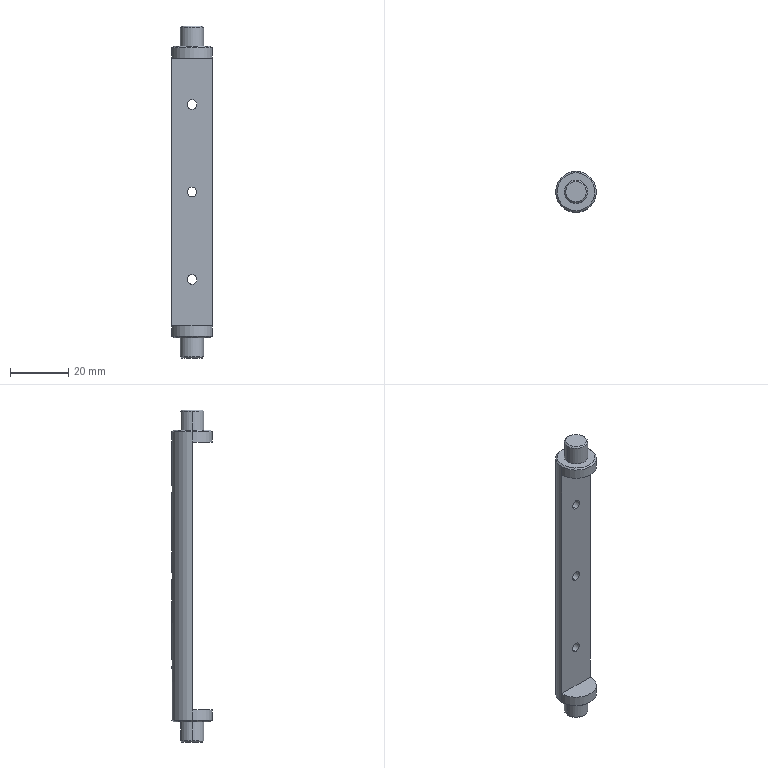Part | STEP file | 2056 Blade rotary shaft | 1 solid | 28 faces | box 14 x 14 x 114 mm | volume 8821 mm3 | cylinder 13 | cone 8 | plane 7 | commonest cylinder face diameters 3.3 x6 8 x4 14 x3